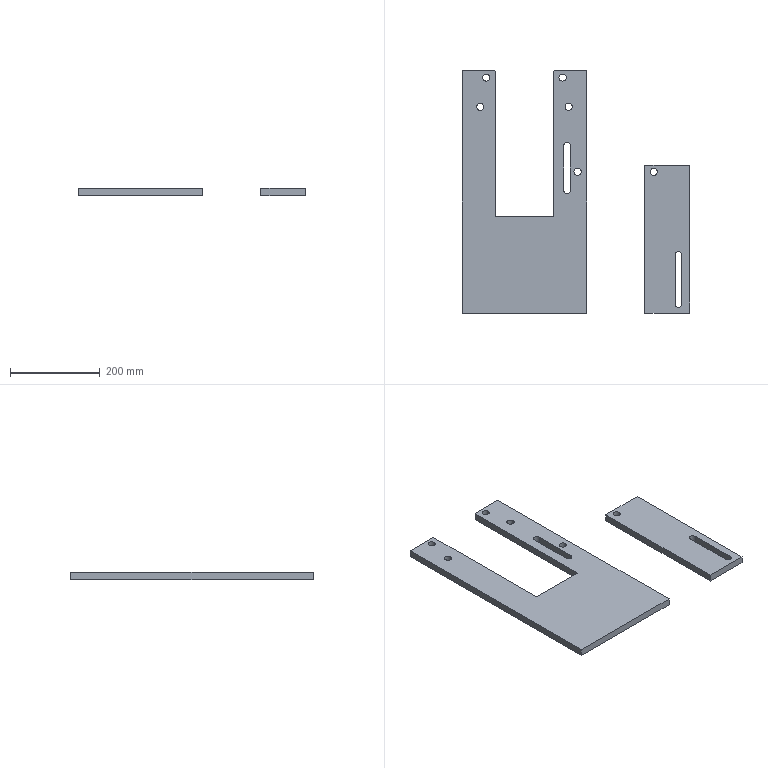Part | STEP file | 2 solids | 38 faces | box 507 x 540 x 16 mm | volume 2169859 mm3 | plane 22 | cylinder 16 | commonest cylinder face diameters 16 x12 15 x4